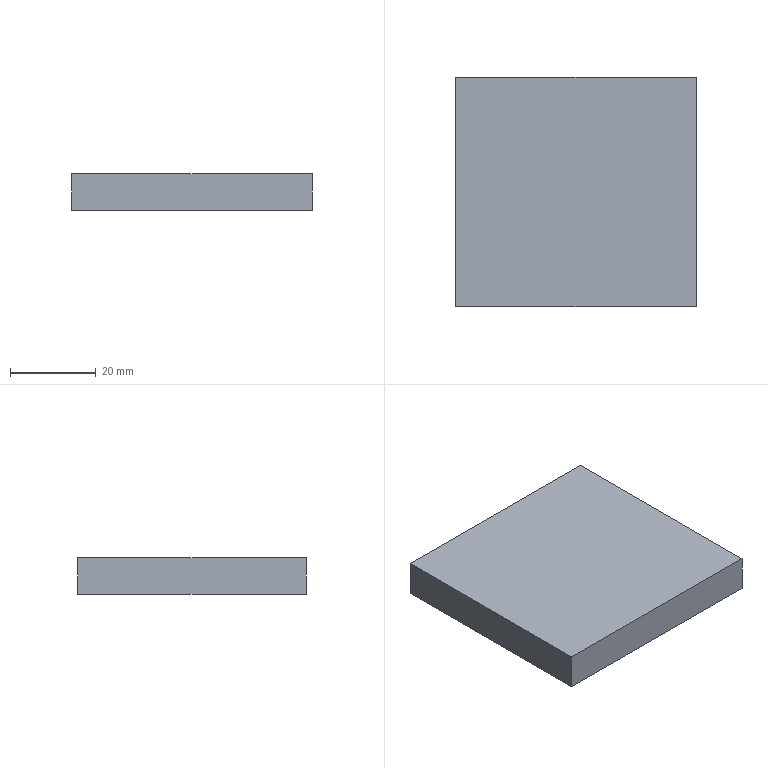NC program | NX | posted with a generic post | part box 56 x 53.3 x 8.5 mm
Lines 590 to 2012 of 2943:
(CAVITY_MILL_COPY_COPY , TOOL : D4)
N1178 T11 M6
N1180 G54
N1182 G17 G0 G90 X-8.53 Y16.809 S9500 M3
N1184 G43 Z30. H11
N1186 Z0.708
N1188 G94 G1 Z-0.292 F800.
N1190 X-8.86 Y16.999
N1192 G3 X-9.86 Y16.997 R1.
N1194 X-10.379 Y16.685 R19.65 F1200.
N1196 X-10.558 Y16.028 R0.5
N1198 G2 X-10.331 Y15.511 R4.05
N1200 G3 X-9.567 Y14.865 R1.
N1202 G1 X-9.34 Y14.824
N1204 Z0.708
N1206 X-8.53 Y16.809 Z0.417 F6000.
N1208 Z-0.583 F800.
N1210 X-8.86 Y16.999
N1212 G3 X-9.86 Y16.997 R1.
N1214 X-10.379 Y16.685 R19.65 F1200.
N1216 X-10.558 Y16.028 R0.5
N1218 G2 X-10.331 Y15.511 R4.05
N1220 G3 X-9.567 Y14.865 R1.
N1222 G1 X-9.34 Y14.824
N1224 Z0.417
N1226 X-8.53 Y16.809 Z0.125 F6000.
N1228 Z-0.875 F800.
N1230 X-8.86 Y16.999
N1232 G3 X-9.86 Y16.997 R1.
N1234 X-10.379 Y16.685 R19.65 F1200.
N1236 X-10.558 Y16.028 R0.5
N1238 G2 X-10.331 Y15.511 R4.05
N1240 G3 X-9.567 Y14.865 R1.
N1242 G1 X-9.34 Y14.824
N1244 Z0.125
N1246 X-8.53 Y16.809 Z-0.167 F6000.
N1248 Z-1.167 F800.
N1250 X-8.86 Y16.999
N1252 G3 X-9.86 Y16.997 R1.
N1254 X-10.379 Y16.685 R19.65 F1200.
N1256 X-10.558 Y16.028 R0.5
N1258 G2 X-10.331 Y15.511 R4.05
N1260 G3 X-9.567 Y14.865 R1.
N1262 G1 X-9.34 Y14.824
N1264 Z-0.167
N1266 X-8.53 Y16.809 Z-0.458 F6000.
N1268 Z-1.458 F800.
N1270 X-8.86 Y16.999
N1272 G3 X-9.86 Y16.997 R1.
N1274 X-10.379 Y16.685 R19.65 F1200.
N1276 X-10.558 Y16.028 R0.5
N1278 G2 X-10.331 Y15.511 R4.05
N1280 G3 X-9.567 Y14.865 R1.
N1282 G1 X-9.34 Y14.824
N1284 Z-0.458
N1286 X-8.53 Y16.809 Z-0.75 F6000.
N1288 Z-1.75 F800.
N1290 X-8.86 Y16.999
N1292 G3 X-9.86 Y16.997 R1.
N1294 X-10.379 Y16.685 R19.65 F1200.
N1296 X-10.558 Y16.028 R0.5
N1298 G2 X-10.331 Y15.511 R4.05
N1300 G3 X-9.567 Y14.865 R1.
N1302 G1 X-9.34 Y14.824
N1304 Z-0.75
N1306 X-8.53 Y16.809 Z-1.042 F6000.
N1308 Z-2.042 F800.
N1310 X-8.86 Y16.999
N1312 G3 X-9.86 Y16.997 R1.
N1314 X-10.379 Y16.685 R19.65 F1200.
N1316 X-10.558 Y16.028 R0.5
N1318 G2 X-10.331 Y15.511 R4.05
N1320 G3 X-9.567 Y14.865 R1.
N1322 G1 X-9.34 Y14.824
N1324 Z-1.042
N1326 X-8.53 Y16.809 Z-1.333 F6000.
N1328 Z-2.333 F800.
N1330 X-8.86 Y16.999
N1332 G3 X-9.86 Y16.997 R1.
N1334 X-10.379 Y16.685 R19.65 F1200.
N1336 X-10.558 Y16.028 R0.5
N1338 G2 X-10.331 Y15.511 R4.05
N1340 G3 X-9.567 Y14.865 R1.
N1342 G1 X-9.34 Y14.824
N1344 Z-1.333
N1346 X-8.53 Y16.809 Z-1.625 F6000.
N1348 Z-2.625 F800.
N1350 X-8.86 Y16.999
N1352 G3 X-9.86 Y16.997 R1.
N1354 X-10.379 Y16.685 R19.65 F1200.
N1356 X-10.558 Y16.028 R0.5
N1358 G2 X-10.331 Y15.511 R4.05
N1360 G3 X-9.567 Y14.865 R1.
N1362 G1 X-9.34 Y14.824
N1364 Z-1.625
N1366 X-8.53 Y16.809 Z-1.917 F6000.
N1368 Z-2.917 F800.
N1370 X-8.86 Y16.999
N1372 G3 X-9.86 Y16.997 R1.
N1374 X-10.379 Y16.685 R19.65 F1200.
N1376 X-10.558 Y16.028 R0.5
N1378 G2 X-10.331 Y15.511 R4.05
N1380 G3 X-9.567 Y14.865 R1.
N1382 G1 X-9.34 Y14.824
N1384 Z-1.917
N1386 X-8.53 Y16.809 Z-2.208 F6000.
N1388 Z-3.208 F800.
N1390 X-8.86 Y16.999
N1392 G3 X-9.86 Y16.997 R1.
N1394 X-10.379 Y16.685 R19.65 F1200.
N1396 X-10.558 Y16.028 R0.5
N1398 G2 X-10.331 Y15.511 R4.05
N1400 G3 X-9.567 Y14.865 R1.
N1402 G1 X-9.34 Y14.824
N1404 Z-2.208
N1406 X-8.53 Y16.809 Z-2.5 F6000.
N1408 Z-3.5 F800.
N1410 X-8.86 Y16.999
N1412 G3 X-9.86 Y16.997 R1.
N1414 X-10.379 Y16.685 R19.65 F1200.
N1416 X-10.558 Y16.028 R0.5
N1418 G2 X-10.331 Y15.511 R4.05
N1420 G3 X-9.567 Y14.865 R1.
N1422 G1 X-9.34 Y14.824
N1424 Z-2.5
N1426 G0 Z30.
N1428 X-14.824 Y9.34
N1430 Z0.708
N1432 G1 Z-0.292 F800.
N1434 X-14.865 Y9.567
N1436 G3 X-15.511 Y10.331 R1.
N1438 G2 X-16.028 Y10.558 R4.05 F1200.
N1440 G3 X-16.685 Y10.379 R0.5
N1442 X-16.997 Y9.86 R19.65
N1444 X-16.999 Y8.86 R1.
N1446 G1 X-16.809 Y8.53
N1448 Z0.708
N1450 X-14.824 Y9.34 Z0.417 F6000.
N1452 Z-0.583 F800.
N1454 X-14.865 Y9.567
N1456 G3 X-15.511 Y10.331 R1.
N1458 G2 X-16.028 Y10.558 R4.05 F1200.
N1460 G3 X-16.685 Y10.379 R0.5
N1462 X-16.997 Y9.86 R19.65
N1464 X-16.999 Y8.86 R1.
N1466 G1 X-16.809 Y8.53
N1468 Z0.417
N1470 X-14.824 Y9.34 Z0.125 F6000.
N1472 Z-0.875 F800.
N1474 X-14.865 Y9.567
N1476 G3 X-15.511 Y10.331 R1.
N1478 G2 X-16.028 Y10.558 R4.05 F1200.
N1480 G3 X-16.685 Y10.379 R0.5
N1482 X-16.997 Y9.86 R19.65
N1484 X-16.999 Y8.86 R1.
N1486 G1 X-16.809 Y8.53
N1488 Z0.125
N1490 X-14.824 Y9.34 Z-0.167 F6000.
N1492 Z-1.167 F800.
N1494 X-14.865 Y9.567
N1496 G3 X-15.511 Y10.331 R1.
N1498 G2 X-16.028 Y10.558 R4.05 F1200.
N1500 G3 X-16.685 Y10.379 R0.5
N1502 X-16.997 Y9.86 R19.65
N1504 X-16.999 Y8.86 R1.
N1506 G1 X-16.809 Y8.53
N1508 Z-0.167
N1510 X-14.824 Y9.34 Z-0.458 F6000.
N1512 Z-1.458 F800.
N1514 X-14.865 Y9.567
N1516 G3 X-15.511 Y10.331 R1.
N1518 G2 X-16.028 Y10.558 R4.05 F1200.
N1520 G3 X-16.685 Y10.379 R0.5
N1522 X-16.997 Y9.86 R19.65
N1524 X-16.999 Y8.86 R1.
N1526 G1 X-16.809 Y8.53
N1528 Z-0.458
N1530 X-14.824 Y9.34 Z-0.75 F6000.
N1532 Z-1.75 F800.
N1534 X-14.865 Y9.567
N1536 G3 X-15.511 Y10.331 R1.
N1538 G2 X-16.028 Y10.558 R4.05 F1200.
N1540 G3 X-16.685 Y10.379 R0.5
N1542 X-16.997 Y9.86 R19.65
N1544 X-16.999 Y8.86 R1.
N1546 G1 X-16.809 Y8.53
N1548 Z-0.75
N1550 X-14.824 Y9.34 Z-1.042 F6000.
N1552 Z-2.042 F800.
N1554 X-14.865 Y9.567
N1556 G3 X-15.511 Y10.331 R1.
N1558 G2 X-16.028 Y10.558 R4.05 F1200.
N1560 G3 X-16.685 Y10.379 R0.5
N1562 X-16.997 Y9.86 R19.65
N1564 X-16.999 Y8.86 R1.
N1566 G1 X-16.809 Y8.53
N1568 Z-1.042
N1570 X-14.824 Y9.34 Z-1.333 F6000.
N1572 Z-2.333 F800.
N1574 X-14.865 Y9.567
N1576 G3 X-15.511 Y10.331 R1.
N1578 G2 X-16.028 Y10.558 R4.05 F1200.
N1580 G3 X-16.685 Y10.379 R0.5
N1582 X-16.997 Y9.86 R19.65
N1584 X-16.999 Y8.86 R1.
N1586 G1 X-16.809 Y8.53
N1588 Z-1.333
N1590 X-14.824 Y9.34 Z-1.625 F6000.
N1592 Z-2.625 F800.
N1594 X-14.865 Y9.567
N1596 G3 X-15.511 Y10.331 R1.
N1598 G2 X-16.028 Y10.558 R4.05 F1200.
N1600 G3 X-16.685 Y10.379 R0.5
N1602 X-16.997 Y9.86 R19.65
N1604 X-16.999 Y8.86 R1.
N1606 G1 X-16.809 Y8.53
N1608 Z-1.625
N1610 X-14.824 Y9.34 Z-1.917 F6000.
N1612 Z-2.917 F800.
N1614 X-14.865 Y9.567
N1616 G3 X-15.511 Y10.331 R1.
N1618 G2 X-16.028 Y10.558 R4.05 F1200.
N1620 G3 X-16.685 Y10.379 R0.5
N1622 X-16.997 Y9.86 R19.65
N1624 X-16.999 Y8.86 R1.
N1626 G1 X-16.809 Y8.53
N1628 Z-1.917
N1630 X-14.824 Y9.34 Z-2.208 F6000.
N1632 Z-3.208 F800.
N1634 X-14.865 Y9.567
N1636 G3 X-15.511 Y10.331 R1.
N1638 G2 X-16.028 Y10.558 R4.05 F1200.
N1640 G3 X-16.685 Y10.379 R0.5
N1642 X-16.997 Y9.86 R19.65
N1644 X-16.999 Y8.86 R1.
N1646 G1 X-16.809 Y8.53
N1648 Z-2.208
N1650 X-14.824 Y9.34 Z-2.5 F6000.
N1652 Z-3.5 F800.
N1654 X-14.865 Y9.567
N1656 G3 X-15.511 Y10.331 R1.
N1658 G2 X-16.028 Y10.558 R4.05 F1200.
N1660 G3 X-16.685 Y10.379 R0.5
N1662 X-16.997 Y9.86 R19.65
N1664 X-16.999 Y8.86 R1.
N1666 G1 X-16.809 Y8.53
N1668 Z-2.5
N1670 G0 Z30.
N1672 X-18.46 Y5.669
N1674 Z0.708
N1676 G1 Z-0.292 F800.
N1678 X-18.629 Y5.779
N1680 G3 X-19.628 Y5.829 R1.
N1682 G2 X-20.241 Y5.596 R3. F1200.
N1684 G3 X-20.412 Y4.934 R21.
N1686 X-20.13 Y3.974 R1.
N1688 G1 X-19.856 Y3.713
N1690 Z0.708
N1692 X-18.46 Y5.669 Z0.417 F6000.
N1694 Z-0.583 F800.
N1696 X-18.629 Y5.779
N1698 G3 X-19.628 Y5.829 R1.
N1700 G2 X-20.241 Y5.596 R3. F1200.
N1702 G3 X-20.412 Y4.934 R21.
N1704 X-20.13 Y3.974 R1.
N1706 G1 X-19.856 Y3.713
N1708 Z0.417
N1710 X-18.46 Y5.669 Z0.125 F6000.
N1712 Z-0.875 F800.
N1714 X-18.629 Y5.779
N1716 G3 X-19.628 Y5.829 R1.
N1718 G2 X-20.241 Y5.596 R3. F1200.
N1720 G3 X-20.412 Y4.934 R21.
N1722 X-20.13 Y3.974 R1.
N1724 G1 X-19.856 Y3.713
N1726 Z0.125
N1728 X-18.46 Y5.669 Z-0.167 F6000.
N1730 Z-1.167 F800.
N1732 X-18.629 Y5.779
N1734 G3 X-19.628 Y5.829 R1.
N1736 G2 X-20.241 Y5.596 R3. F1200.
N1738 G3 X-20.412 Y4.934 R21.
N1740 X-20.13 Y3.974 R1.
N1742 G1 X-19.856 Y3.713
N1744 Z-0.167
N1746 X-18.46 Y5.669 Z-0.458 F6000.
N1748 Z-1.458 F800.
N1750 X-18.629 Y5.779
N1752 G3 X-19.628 Y5.829 R1.
N1754 G2 X-20.241 Y5.596 R3. F1200.
N1756 G3 X-20.412 Y4.934 R21.
N1758 X-20.13 Y3.974 R1.
N1760 G1 X-19.856 Y3.713
N1762 Z-0.458
N1764 X-18.46 Y5.669 Z-0.75 F6000.
N1766 Z-1.75 F800.
N1768 X-18.629 Y5.779
N1770 G3 X-19.628 Y5.829 R1.
N1772 G2 X-20.241 Y5.596 R3. F1200.
N1774 G3 X-20.412 Y4.934 R21.
N1776 X-20.13 Y3.974 R1.
N1778 G1 X-19.856 Y3.713
N1780 Z-0.75
N1782 X-18.46 Y5.669 Z-1.042 F6000.
N1784 Z-2.042 F800.
N1786 X-18.629 Y5.779
N1788 G3 X-19.628 Y5.829 R1.
N1790 G2 X-20.241 Y5.596 R3. F1200.
N1792 G3 X-20.412 Y4.934 R21.
N1794 X-20.13 Y3.974 R1.
N1796 G1 X-19.856 Y3.713
N1798 Z-1.042
N1800 X-18.46 Y5.669 Z-1.333 F6000.
N1802 Z-2.333 F800.
N1804 X-18.629 Y5.779
N1806 G3 X-19.628 Y5.829 R1.
N1808 G2 X-20.241 Y5.596 R3. F1200.
N1810 G3 X-20.412 Y4.934 R21.
N1812 X-20.13 Y3.974 R1.
N1814 G1 X-19.856 Y3.713
N1816 Z-1.333
N1818 X-18.46 Y5.669 Z-1.625 F6000.
N1820 Z-2.625 F800.
N1822 X-18.629 Y5.779
N1824 G3 X-19.628 Y5.829 R1.
N1826 G2 X-20.241 Y5.596 R3. F1200.
N1828 G3 X-20.412 Y4.934 R21.
N1830 X-20.13 Y3.974 R1.
N1832 G1 X-19.856 Y3.713
N1834 Z-1.625
N1836 X-18.46 Y5.669 Z-1.917 F6000.
N1838 Z-2.917 F800.
N1840 X-18.629 Y5.779
N1842 G3 X-19.628 Y5.829 R1.
N1844 G2 X-20.241 Y5.596 R3. F1200.
N1846 G3 X-20.412 Y4.934 R21.
N1848 X-20.13 Y3.974 R1.
N1850 G1 X-19.856 Y3.713
N1852 Z-1.917
N1854 X-18.46 Y5.669 Z-2.208 F6000.
N1856 Z-3.208 F800.
N1858 X-18.629 Y5.779
N1860 G3 X-19.628 Y5.829 R1.
N1862 G2 X-20.241 Y5.596 R3. F1200.
N1864 G3 X-20.412 Y4.934 R21.
N1866 X-20.13 Y3.974 R1.
N1868 G1 X-19.856 Y3.713
N1870 Z-2.208
N1872 X-18.46 Y5.669 Z-2.5 F6000.
N1874 Z-3.5 F800.
N1876 X-18.629 Y5.779
N1878 G3 X-19.628 Y5.829 R1.
N1880 G2 X-20.241 Y5.596 R3. F1200.
N1882 G3 X-20.412 Y4.934 R21.
N1884 X-20.13 Y3.974 R1.
N1886 G1 X-19.856 Y3.713
N1888 Z-2.5
N1890 G0 Z30.
N1892 Y-3.713
N1894 Z0.708
N1896 G1 Z-0.292 F800.
N1898 X-20.13 Y-3.974
N1900 G3 X-20.412 Y-4.934 R1.
N1902 X-20.241 Y-5.596 R21. F1200.
N1904 G2 X-19.628 Y-5.829 R3.
N1906 G3 X-18.629 Y-5.779 R1.
N1908 G1 X-18.46 Y-5.669
N1910 Z0.708
N1912 X-19.856 Y-3.713 Z0.417 F6000.
N1914 Z-0.583 F800.
N1916 X-20.13 Y-3.974
N1918 G3 X-20.412 Y-4.934 R1.
N1920 X-20.241 Y-5.596 R21. F1200.
N1922 G2 X-19.628 Y-5.829 R3.
N1924 G3 X-18.629 Y-5.779 R1.
N1926 G1 X-18.46 Y-5.669
N1928 Z0.417
N1930 X-19.856 Y-3.713 Z0.125 F6000.
N1932 Z-0.875 F800.
N1934 X-20.13 Y-3.974
N1936 G3 X-20.412 Y-4.934 R1.
N1938 X-20.241 Y-5.596 R21. F1200.
N1940 G2 X-19.628 Y-5.829 R3.
N1942 G3 X-18.629 Y-5.779 R1.
N1944 G1 X-18.46 Y-5.669
N1946 Z0.125
N1948 X-19.856 Y-3.713 Z-0.167 F6000.
N1950 Z-1.167 F800.
N1952 X-20.13 Y-3.974
N1954 G3 X-20.412 Y-4.934 R1.
N1956 X-20.241 Y-5.596 R21. F1200.
N1958 G2 X-19.628 Y-5.829 R3.
N1960 G3 X-18.629 Y-5.779 R1.
N1962 G1 X-18.46 Y-5.669
N1964 Z-0.167
N1966 X-19.856 Y-3.713 Z-0.458 F6000.
N1968 Z-1.458 F800.
N1970 X-20.13 Y-3.974
N1972 G3 X-20.412 Y-4.934 R1.
N1974 X-20.241 Y-5.596 R21. F1200.
N1976 G2 X-19.628 Y-5.829 R3.
N1978 G3 X-18.629 Y-5.779 R1.
N1980 G1 X-18.46 Y-5.669
N1982 Z-0.458
N1984 X-19.856 Y-3.713 Z-0.75 F6000.
N1986 Z-1.75 F800.
N1988 X-20.13 Y-3.974
N1990 G3 X-20.412 Y-4.934 R1.
N1992 X-20.241 Y-5.596 R21. F1200.
N1994 G2 X-19.628 Y-5.829 R3.
N1996 G3 X-18.629 Y-5.779 R1.
N1998 G1 X-18.46 Y-5.669
N2000 Z-0.75
N2002 X-19.856 Y-3.713 Z-1.042 F6000.
N2004 Z-2.042 F800.
N2006 X-20.13 Y-3.974
N2008 G3 X-20.412 Y-4.934 R1.
N2010 X-20.241 Y-5.596 R21. F1200.
N2012 G2 X-19.628 Y-5.829 R3.
N2014 G3 X-18.629 Y-5.779 R1.
N2016 G1 X-18.46 Y-5.669
N2018 Z-1.042
N2020 X-19.856 Y-3.713 Z-1.333 F6000.
N2022 Z-2.333 F800.
N2024 X-20.13 Y-3.974
N2026 G3 X-20.412 Y-4.934 R1.
N2028 X-20.241 Y-5.596 R21. F1200.
N2030 G2 X-19.628 Y-5.829 R3.
N2032 G3 X-18.629 Y-5.779 R1.
N2034 G1 X-18.46 Y-5.669
N2036 Z-1.333
N2038 X-19.856 Y-3.713 Z-1.625 F6000.
N2040 Z-2.625 F800.
N2042 X-20.13 Y-3.974
N2044 G3 X-20.412 Y-4.934 R1.
N2046 X-20.241 Y-5.596 R21. F1200.
N2048 G2 X-19.628 Y-5.829 R3.
N2050 G3 X-18.629 Y-5.779 R1.
N2052 G1 X-18.46 Y-5.669
N2054 Z-1.625
N2056 X-19.856 Y-3.713 Z-1.917 F6000.
N2058 Z-2.917 F800.
N2060 X-20.13 Y-3.974
N2062 G3 X-20.412 Y-4.934 R1.
N2064 X-20.241 Y-5.596 R21. F1200.
N2066 G2 X-19.628 Y-5.829 R3.
N2068 G3 X-18.629 Y-5.779 R1.
N2070 G1 X-18.46 Y-5.669
N2072 Z-1.917
N2074 X-19.856 Y-3.713 Z-2.208 F6000.
N2076 Z-3.208 F800.
N2078 X-20.13 Y-3.974
N2080 G3 X-20.412 Y-4.934 R1.
N2082 X-20.241 Y-5.596 R21. F1200.
N2084 G2 X-19.628 Y-5.829 R3.
N2086 G3 X-18.629 Y-5.779 R1.
N2088 G1 X-18.46 Y-5.669
N2090 Z-2.208
N2092 X-19.856 Y-3.713 Z-2.5 F6000.
N2094 Z-3.5 F800.
N2096 X-20.13 Y-3.974
N2098 G3 X-20.412 Y-4.934 R1.
N2100 X-20.241 Y-5.596 R21. F1200.
N2102 G2 X-19.628 Y-5.829 R3.
N2104 G3 X-18.629 Y-5.779 R1.
N2106 G1 X-18.46 Y-5.669
N2108 Z-2.5
N2110 G0 Z30.
N2112 X-16.809 Y-8.53
N2114 Z0.708
N2116 G1 Z-0.292 F800.
N2118 X-16.999 Y-8.86
N2120 G3 X-16.997 Y-9.86 R1.
N2122 X-16.685 Y-10.379 R19.65 F1200.
N2124 X-16.028 Y-10.558 R0.5
N2126 G2 X-15.511 Y-10.331 R4.05
N2128 G3 X-14.865 Y-9.567 R1.
N2130 G1 X-14.824 Y-9.34
N2132 Z0.708
N2134 X-16.809 Y-8.53 Z0.417 F6000.
N2136 Z-0.583 F800.
N2138 X-16.999 Y-8.86
N2140 G3 X-16.997 Y-9.86 R1.
N2142 X-16.685 Y-10.379 R19.65 F1200.
N2144 X-16.028 Y-10.558 R0.5
N2146 G2 X-15.511 Y-10.331 R4.05
N2148 G3 X-14.865 Y-9.567 R1.
N2150 G1 X-14.824 Y-9.34
N2152 Z0.417
N2154 X-16.809 Y-8.53 Z0.125 F6000.
N2156 Z-0.875 F800.
N2158 X-16.999 Y-8.86
N2160 G3 X-16.997 Y-9.86 R1.
N2162 X-16.685 Y-10.379 R19.65 F1200.
N2164 X-16.028 Y-10.558 R0.5
N2166 G2 X-15.511 Y-10.331 R4.05
N2168 G3 X-14.865 Y-9.567 R1.
N2170 G1 X-14.824 Y-9.34
N2172 Z0.125
N2174 X-16.809 Y-8.53 Z-0.167 F6000.
N2176 Z-1.167 F800.
N2178 X-16.999 Y-8.86
N2180 G3 X-16.997 Y-9.86 R1.
N2182 X-16.685 Y-10.379 R19.65 F1200.
N2184 X-16.028 Y-10.558 R0.5
N2186 G2 X-15.511 Y-10.331 R4.05
N2188 G3 X-14.865 Y-9.567 R1.
N2190 G1 X-14.824 Y-9.34
N2192 Z-0.167
N2194 X-16.809 Y-8.53 Z-0.458 F6000.
N2196 Z-1.458 F800.
N2198 X-16.999 Y-8.86
N2200 G3 X-16.997 Y-9.86 R1.
N2202 X-16.685 Y-10.379 R19.65 F1200.
N2204 X-16.028 Y-10.558 R0.5
N2206 G2 X-15.511 Y-10.331 R4.05
N2208 G3 X-14.865 Y-9.567 R1.
N2210 G1 X-14.824 Y-9.34
N2212 Z-0.458
N2214 X-16.809 Y-8.53 Z-0.75 F6000.
N2216 Z-1.75 F800.
N2218 X-16.999 Y-8.86
N2220 G3 X-16.997 Y-9.86 R1.
N2222 X-16.685 Y-10.379 R19.65 F1200.
N2224 X-16.028 Y-10.558 R0.5
N2226 G2 X-15.511 Y-10.331 R4.05
N2228 G3 X-14.865 Y-9.567 R1.
N2230 G1 X-14.824 Y-9.34
N2232 Z-0.75
N2234 X-16.809 Y-8.53 Z-1.042 F6000.
N2236 Z-2.042 F800.
N2238 X-16.999 Y-8.86
N2240 G3 X-16.997 Y-9.86 R1.
N2242 X-16.685 Y-10.379 R19.65 F1200.
N2244 X-16.028 Y-10.558 R0.5
N2246 G2 X-15.511 Y-10.331 R4.05
N2248 G3 X-14.865 Y-9.567 R1.
N2250 G1 X-14.824 Y-9.34
N2252 Z-1.042
N2254 X-16.809 Y-8.53 Z-1.333 F6000.
N2256 Z-2.333 F800.
N2258 X-16.999 Y-8.86
N2260 G3 X-16.997 Y-9.86 R1.
N2262 X-16.685 Y-10.379 R19.65 F1200.
N2264 X-16.028 Y-10.558 R0.5
N2266 G2 X-15.511 Y-10.331 R4.05
N2268 G3 X-14.865 Y-9.567 R1.
N2270 G1 X-14.824 Y-9.34
N2272 Z-1.333
N2274 X-16.809 Y-8.53 Z-1.625 F6000.
N2276 Z-2.625 F800.
N2278 X-16.999 Y-8.86
N2280 G3 X-16.997 Y-9.86 R1.
N2282 X-16.685 Y-10.379 R19.65 F1200.
N2284 X-16.028 Y-10.558 R0.5
N2286 G2 X-15.511 Y-10.331 R4.05
N2288 G3 X-14.865 Y-9.567 R1.
N2290 G1 X-14.824 Y-9.34
N2292 Z-1.625
N2294 X-16.809 Y-8.53 Z-1.917 F6000.
N2296 Z-2.917 F800.
N2298 X-16.999 Y-8.86
N2300 G3 X-16.997 Y-9.86 R1.
N2302 X-16.685 Y-10.379 R19.65 F1200.
N2304 X-16.028 Y-10.558 R0.5
N2306 G2 X-15.511 Y-10.331 R4.05
N2308 G3 X-14.865 Y-9.567 R1.
N2310 G1 X-14.824 Y-9.34
N2312 Z-1.917
N2314 X-16.809 Y-8.53 Z-2.208 F6000.
N2316 Z-3.208 F800.
N2318 X-16.999 Y-8.86
N2320 G3 X-16.997 Y-9.86 R1.
N2322 X-16.685 Y-10.379 R19.65 F1200.
N2324 X-16.028 Y-10.558 R0.5
N2326 G2 X-15.511 Y-10.331 R4.05
N2328 G3 X-14.865 Y-9.567 R1.
N2330 G1 X-14.824 Y-9.34
N2332 Z-2.208
N2334 X-16.809 Y-8.53 Z-2.5 F6000.
N2336 Z-3.5 F800.
N2338 X-16.999 Y-8.86
N2340 G3 X-16.997 Y-9.86 R1.
N2342 X-16.685 Y-10.379 R19.65 F1200.
N2344 X-16.028 Y-10.558 R0.5
N2346 G2 X-15.511 Y-10.331 R4.05
N2348 G3 X-14.865 Y-9.567 R1.
N2350 G1 X-14.824 Y-9.34
N2352 Z-2.5
N2354 G0 Z30.
N2356 X-9.34 Y-14.824
N2358 Z0.708
N2360 G1 Z-0.292 F800.
N2362 X-9.567 Y-14.865
N2364 G3 X-10.331 Y-15.511 R1.
N2366 G2 X-10.558 Y-16.028 R4.05 F1200.
N2368 G3 X-10.379 Y-16.685 R0.5
N2370 X-9.86 Y-16.997 R19.65
N2372 X-8.86 Y-16.999 R1.
N2374 G1 X-8.53 Y-16.809
N2376 Z0.708
N2378 X-9.34 Y-14.824 Z0.417 F6000.
N2380 Z-0.583 F800.
N2382 X-9.567 Y-14.865
N2384 G3 X-10.331 Y-15.511 R1.
N2386 G2 X-10.558 Y-16.028 R4.05 F1200.
N2388 G3 X-10.379 Y-16.685 R0.5
N2390 X-9.86 Y-16.997 R19.65
N2392 X-8.86 Y-16.999 R1.
N2394 G1 X-8.53 Y-16.81
N2396 Z0.417
N2398 X-9.34 Y-14.824 Z0.125 F6000.
N2400 Z-0.875 F800.
N2402 X-9.567 Y-14.865
N2404 G3 X-10.331 Y-15.511 R1.
N2406 G2 X-10.558 Y-16.028 R4.05 F1200.
N2408 G3 X-10.379 Y-16.685 R0.5
N2410 X-9.86 Y-16.997 R19.65
N2412 X-8.86 Y-16.999 R1.
N2414 G1 X-8.53 Y-16.81
N2416 Z0.125
N2418 X-9.34 Y-14.824 Z-0.167 F6000.
N2420 Z-1.167 F800.
N2422 X-9.567 Y-14.865
N2424 G3 X-10.331 Y-15.511 R1.
N2426 G2 X-10.558 Y-16.028 R4.05 F1200.
N2428 G3 X-10.379 Y-16.685 R0.5
N2430 X-9.86 Y-16.997 R19.65
N2432 X-8.86 Y-16.999 R1.
N2434 G1 X-8.53 Y-16.81
N2436 Z-0.167
N2438 X-9.34 Y-14.824 Z-0.458 F6000.
N2440 Z-1.458 F800.
N2442 X-9.567 Y-14.865
N2444 G3 X-10.33 Y-15.511 R1.
N2446 G2 X-10.558 Y-16.028 R4.05 F1200.
N2448 G3 X-10.379 Y-16.685 R0.5
N2450 X-9.86 Y-16.997 R19.65
N2452 X-8.86 Y-16.999 R1.
N2454 G1 X-8.53 Y-16.81
N2456 Z-0.458
N2458 X-9.34 Y-14.824 Z-0.75 F6000.
N2460 Z-1.75 F800.
N2462 X-9.567 Y-14.865
N2464 G3 X-10.33 Y-15.511 R1.
N2466 G2 X-10.558 Y-16.028 R4.05 F1200.
N2468 G3 X-10.379 Y-16.685 R0.5
N2470 X-9.86 Y-16.997 R19.65
N2472 X-8.86 Y-16.999 R1.
N2474 G1 X-8.53 Y-16.81
N2476 Z-0.75
N2478 X-9.34 Y-14.824 Z-1.042 F6000.
N2480 Z-2.042 F800.
N2482 X-9.567 Y-14.865
N2484 G3 X-10.33 Y-15.511 R1.
N2486 G2 X-10.558 Y-16.028 R4.05 F1200.
N2488 G3 X-10.379 Y-16.685 R0.5
N2490 X-9.86 Y-16.997 R19.65
N2492 X-8.86 Y-16.999 R1.
N2494 G1 X-8.53 Y-16.81
N2496 Z-1.042
N2498 X-9.34 Y-14.824 Z-1.333 F6000.
N2500 Z-2.333 F800.
N2502 X-9.567 Y-14.865
N2504 G3 X-10.33 Y-15.511 R1.
N2506 G2 X-10.558 Y-16.028 R4.05 F1200.
N2508 G3 X-10.379 Y-16.685 R0.5
N2510 X-9.86 Y-16.997 R19.65
N2512 X-8.86 Y-16.999 R1.
N2514 G1 X-8.53 Y-16.81
N2516 Z-1.333
N2518 X-9.34 Y-14.823 Z-1.625 F6000.
N2520 Z-2.625 F800.
N2522 X-9.567 Y-14.864
N2524 G3 X-10.33 Y-15.511 R1.
N2526 G2 X-10.558 Y-16.028 R4.05 F1200.
N2528 G3 X-10.379 Y-16.685 R0.5
N2530 X-9.859 Y-16.997 R19.65
N2532 X-8.859 Y-16.999 R1.
N2534 G1 X-8.529 Y-16.81
N2536 Z-1.625
N2538 X-9.34 Y-14.823 Z-1.917 F6000.
N2540 Z-2.917 F800.
N2542 X-9.567 Y-14.864
N2544 G3 X-10.33 Y-15.511 R1.
N2546 G2 X-10.558 Y-16.028 R4.05 F1200.
N2548 G3 X-10.379 Y-16.685 R0.5
N2550 X-9.859 Y-16.998 R19.65
N2552 X-8.859 Y-17. R1.
N2554 G1 X-8.529 Y-16.81
N2556 Z-1.917
N2558 X-9.34 Y-14.823 Z-2.208 F6000.
N2560 Z-3.208 F800.
N2562 X-9.567 Y-14.864
N2564 G3 X-10.33 Y-15.51 R1.
N2566 G2 X-10.558 Y-16.028 R4.05 F1200.
N2568 G3 X-10.379 Y-16.685 R0.5
N2570 X-9.859 Y-16.998 R19.65
N2572 X-8.859 Y-17. R1.
N2574 G1 X-8.529 Y-16.81
N2576 Z-2.208
N2578 X-9.34 Y-14.823 Z-2.5 F6000.
N2580 Z-3.5 F800.
N2582 X-9.567 Y-14.864
N2584 G3 X-10.33 Y-15.51 R1.
N2586 G2 X-10.558 Y-16.028 R4.05 F1200.
N2588 G3 X-10.379 Y-16.685 R0.5
N2590 X-9.859 Y-16.998 R19.65
N2592 X-8.859 Y-17. R1.
N2594 G1 X-8.529 Y-16.81
N2596 Z-2.5
N2598 G0 Z30.
N2600 X8.53 Y-16.809
N2602 Z0.708
N2604 G1 Z-0.292 F800.
N2606 X8.86 Y-16.999
N2608 G3 X9.86 Y-16.997 R1.
N2610 X10.379 Y-16.685 R19.65 F1200.
N2612 X10.558 Y-16.028 R0.5
N2614 G2 X10.331 Y-15.511 R4.05
N2616 G3 X9.567 Y-14.865 R1.
N2618 G1 X9.34 Y-14.824
N2620 Z0.708
N2622 X8.53 Y-16.809 Z0.417 F6000.
N2624 Z-0.583 F800.
N2626 X8.86 Y-16.999
N2628 G3 X9.86 Y-16.997 R1.
N2630 X10.379 Y-16.685 R19.65 F1200.
N2632 X10.558 Y-16.028 R0.5
N2634 G2 X10.331 Y-15.511 R4.05
N2636 G3 X9.567 Y-14.865 R1.
N2638 G1 X9.34 Y-14.824
N2640 Z0.417
N2642 X8.53 Y-16.809 Z0.125 F6000.
N2644 Z-0.875 F800.
N2646 X8.86 Y-16.999
N2648 G3 X9.86 Y-16.997 R1.
N2650 X10.379 Y-16.685 R19.65 F1200.
N2652 X10.558 Y-16.028 R0.5
N2654 G2 X10.331 Y-15.511 R4.05
N2656 G3 X9.567 Y-14.865 R1.
N2658 G1 X9.34 Y-14.824
N2660 Z0.125
N2662 X8.53 Y-16.809 Z-0.167 F6000.
N2664 Z-1.167 F800.
N2666 X8.86 Y-16.999
N2668 G3 X9.86 Y-16.997 R1.
N2670 X10.379 Y-16.685 R19.65 F1200.
N2672 X10.558 Y-16.028 R0.5
N2674 G2 X10.331 Y-15.511 R4.05
N2676 G3 X9.567 Y-14.865 R1.
N2678 G1 X9.34 Y-14.824
N2680 Z-0.167
N2682 X8.53 Y-16.809 Z-0.458 F6000.
N2684 Z-1.458 F800.
N2686 X8.86 Y-16.999
N2688 G3 X9.86 Y-16.997 R1.
N2690 X10.379 Y-16.685 R19.65 F1200.
N2692 X10.558 Y-16.028 R0.5
N2694 G2 X10.331 Y-15.511 R4.05
N2696 G3 X9.567 Y-14.865 R1.
N2698 G1 X9.34 Y-14.824
N2700 Z-0.458
N2702 X8.53 Y-16.809 Z-0.75 F6000.
N2704 Z-1.75 F800.
N2706 X8.86 Y-16.999
N2708 G3 X9.86 Y-16.997 R1.
N2710 X10.379 Y-16.685 R19.65 F1200.
N2712 X10.558 Y-16.028 R0.5
N2714 G2 X10.331 Y-15.511 R4.05
N2716 G3 X9.567 Y-14.865 R1.
N2718 G1 X9.34 Y-14.824
N2720 Z-0.75
N2722 X8.53 Y-16.809 Z-1.042 F6000.
N2724 Z-2.042 F800.
N2726 X8.86 Y-16.999
N2728 G3 X9.86 Y-16.997 R1.
N2730 X10.379 Y-16.685 R19.65 F1200.
N2732 X10.558 Y-16.028 R0.5
N2734 G2 X10.331 Y-15.511 R4.05
N2736 G3 X9.567 Y-14.865 R1.
N2738 G1 X9.34 Y-14.824
N2740 Z-1.042
N2742 X8.53 Y-16.809 Z-1.333 F6000.
N2744 Z-2.333 F800.
N2746 X8.86 Y-16.999
N2748 G3 X9.86 Y-16.997 R1.
N2750 X10.379 Y-16.685 R19.65 F1200.
N2752 X10.558 Y-16.028 R0.5
N2754 G2 X10.331 Y-15.511 R4.05
N2756 G3 X9.567 Y-14.865 R1.
N2758 G1 X9.34 Y-14.824
N2760 Z-1.333
N2762 X8.53 Y-16.809 Z-1.625 F6000.
N2764 Z-2.625 F800.
N2766 X8.86 Y-16.999
N2768 G3 X9.86 Y-16.997 R1.
N2770 X10.379 Y-16.685 R19.65 F1200.
N2772 X10.558 Y-16.028 R0.5
N2774 G2 X10.331 Y-15.511 R4.05
N2776 G3 X9.567 Y-14.865 R1.
N2778 G1 X9.34 Y-14.824
N2780 Z-1.625
N2782 X8.53 Y-16.809 Z-1.917 F6000.
N2784 Z-2.917 F800.
N2786 X8.86 Y-16.999
N2788 G3 X9.86 Y-16.997 R1.
N2790 X10.379 Y-16.685 R19.65 F1200.
N2792 X10.558 Y-16.028 R0.5
N2794 G2 X10.331 Y-15.511 R4.05
N2796 G3 X9.567 Y-14.865 R1.
N2798 G1 X9.34 Y-14.824
N2800 Z-1.917
N2802 X8.53 Y-16.809 Z-2.208 F6000.
N2804 Z-3.208 F800.
N2806 X8.86 Y-16.999
N2808 G3 X9.86 Y-16.997 R1.
N2810 X10.379 Y-16.685 R19.65 F1200.
N2812 X10.558 Y-16.028 R0.5
N2814 G2 X10.331 Y-15.511 R4.05
N2816 G3 X9.567 Y-14.865 R1.
N2818 G1 X9.34 Y-14.824
N2820 Z-2.208
N2822 X8.53 Y-16.809 Z-2.5 F6000.
N2824 Z-3.5 F800.
N2826 X8.86 Y-16.999
N2828 G3 X9.86 Y-16.997 R1.
N2830 X10.379 Y-16.685 R19.65 F1200.
N2832 X10.558 Y-16.028 R0.5
N2834 G2 X10.331 Y-15.511 R4.05
N2836 G3 X9.567 Y-14.865 R1.
N2838 G1 X9.34 Y-14.824
N2840 Z-2.5
N2842 G0 Z30.
N2844 X14.824 Y-9.34
N2846 Z0.708
N2848 G1 Z-0.292 F800.
N2850 X14.865 Y-9.567
N2852 G3 X15.511 Y-10.331 R1.
N2854 G2 X16.028 Y-10.558 R4.05 F1200.
N2856 G3 X16.685 Y-10.379 R0.5
N2858 X16.997 Y-9.86 R19.65
N2860 X16.999 Y-8.86 R1.
N2862 G1 X16.809 Y-8.53
N2864 Z0.708
N2866 X14.824 Y-9.34 Z0.417 F6000.
N2868 Z-0.583 F800.
N2870 X14.865 Y-9.567
N2872 G3 X15.511 Y-10.331 R1.
N2874 G2 X16.028 Y-10.558 R4.05 F1200.
N2876 G3 X16.685 Y-10.379 R0.5
N2878 X16.997 Y-9.86 R19.65
N2880 X16.999 Y-8.86 R1.
N2882 G1 X16.809 Y-8.53
N2884 Z0.417
N2886 X14.824 Y-9.34 Z0.125 F6000.
N2888 Z-0.875 F800.
N2890 X14.865 Y-9.567
N2892 G3 X15.511 Y-10.331 R1.
N2894 G2 X16.028 Y-10.558 R4.05 F1200.
N2896 G3 X16.685 Y-10.379 R0.5
N2898 X16.997 Y-9.86 R19.65
N2900 X16.999 Y-8.86 R1.
N2902 G1 X16.809 Y-8.53
N2904 Z0.125
N2906 X14.824 Y-9.34 Z-0.167 F6000.
N2908 Z-1.167 F800.
N2910 X14.865 Y-9.567
N2912 G3 X15.511 Y-10.331 R1.
N2914 G2 X16.028 Y-10.558 R4.05 F1200.
N2916 G3 X16.685 Y-10.379 R0.5
N2918 X16.997 Y-9.86 R19.65
N2920 X16.999 Y-8.86 R1.
N2922 G1 X16.809 Y-8.53
N2924 Z-0.167
N2926 X14.824 Y-9.34 Z-0.458 F6000.
N2928 Z-1.458 F800.
N2930 X14.865 Y-9.567
N2932 G3 X15.511 Y-10.331 R1.
N2934 G2 X16.028 Y-10.558 R4.05 F1200.
N2936 G3 X16.685 Y-10.379 R0.5
N2938 X16.997 Y-9.86 R19.65
N2940 X16.999 Y-8.86 R1.
N2942 G1 X16.809 Y-8.53
N2944 Z-0.458
N2946 X14.824 Y-9.34 Z-0.75 F6000.
N2948 Z-1.75 F800.
N2950 X14.865 Y-9.567
N2952 G3 X15.511 Y-10.331 R1.
N2954 G2 X16.028 Y-10.558 R4.05 F1200.
N2956 G3 X16.685 Y-10.379 R0.5
N2958 X16.997 Y-9.86 R19.65
N2960 X16.999 Y-8.86 R1.
N2962 G1 X16.809 Y-8.53
N2964 Z-0.75
N2966 X14.824 Y-9.34 Z-1.042 F6000.
N2968 Z-2.042 F800.
N2970 X14.865 Y-9.567
N2972 G3 X15.511 Y-10.331 R1.
N2974 G2 X16.028 Y-10.558 R4.05 F1200.
N2976 G3 X16.685 Y-10.379 R0.5
N2978 X16.997 Y-9.86 R19.65
N2980 X16.999 Y-8.86 R1.
N2982 G1 X16.809 Y-8.53
N2984 Z-1.042
N2986 X14.824 Y-9.34 Z-1.333 F6000.
N2988 Z-2.333 F800.
N2990 X14.865 Y-9.567
N2992 G3 X15.511 Y-10.331 R1.
N2994 G2 X16.028 Y-10.558 R4.05 F1200.
N2996 G3 X16.685 Y-10.379 R0.5
N2998 X16.997 Y-9.86 R19.65
N3000 X16.999 Y-8.86 R1.
N3002 G1 X16.809 Y-8.53
N3004 Z-1.333
N3006 X14.824 Y-9.34 Z-1.625 F6000.
N3008 Z-2.625 F800.
N3010 X14.865 Y-9.567
N3012 G3 X15.511 Y-10.331 R1.
N3014 G2 X16.028 Y-10.558 R4.05 F1200.
N3016 G3 X16.685 Y-10.379 R0.5
N3018 X16.997 Y-9.86 R19.65
N3020 X16.999 Y-8.86 R1.
N3022 G1 X16.809 Y-8.53
N3024 Z-1.625
N3026 X14.824 Y-9.34 Z-1.917 F6000.
N3028 Z-2.917 F800.
N3030 X14.865 Y-9.567
N3032 G3 X15.511 Y-10.331 R1.
N3034 G2 X16.028 Y-10.558 R4.05 F1200.
N3036 G3 X16.685 Y-10.379 R0.5
N3038 X16.997 Y-9.86 R19.65
N3040 X16.999 Y-8.86 R1.
N3042 G1 X16.809 Y-8.53
N3044 Z-1.917
N3046 X14.824 Y-9.34 Z-2.208 F6000.
N3048 Z-3.208 F800.
N3050 X14.865 Y-9.567
N3052 G3 X15.511 Y-10.331 R1.
N3054 G2 X16.028 Y-10.558 R4.05 F1200.
N3056 G3 X16.685 Y-10.379 R0.5
N3058 X16.997 Y-9.86 R19.65
N3060 X16.999 Y-8.86 R1.
N3062 G1 X16.809 Y-8.53
N3064 Z-2.208
N3066 X14.824 Y-9.34 Z-2.5 F6000.
N3068 Z-3.5 F800.
N3070 X14.865 Y-9.567
N3072 G3 X15.511 Y-10.331 R1.
N3074 G2 X16.028 Y-10.558 R4.05 F1200.
N3076 G3 X16.685 Y-10.379 R0.5
N3078 X16.997 Y-9.86 R19.65
N3080 X16.999 Y-8.86 R1.
N3082 G1 X16.809 Y-8.53
N3084 Z-2.5
N3086 G0 Z30.
N3088 X18.46 Y-5.669
N3090 Z0.708
N3092 G1 Z-0.292 F800.
N3094 X18.629 Y-5.779
N3096 G3 X19.628 Y-5.829 R1.
N3098 G2 X20.241 Y-5.596 R3. F1200.
N3100 G3 X20.412 Y-4.934 R21.
N3102 X20.13 Y-3.974 R1.
N3104 G1 X19.856 Y-3.713
N3106 Z0.708
N3108 X18.46 Y-5.669 Z0.417 F6000.
N3110 Z-0.583 F800.
N3112 X18.629 Y-5.779
N3114 G3 X19.628 Y-5.829 R1.
N3116 G2 X20.241 Y-5.596 R3. F1200.
N3118 G3 X20.412 Y-4.934 R21.
N3120 X20.13 Y-3.974 R1.
N3122 G1 X19.856 Y-3.713
N3124 Z0.417
N3126 X18.46 Y-5.669 Z0.125 F6000.
N3128 Z-0.875 F800.
N3130 X18.629 Y-5.779
N3132 G3 X19.628 Y-5.829 R1.
N3134 G2 X20.241 Y-5.596 R3. F1200.
N3136 G3 X20.412 Y-4.934 R21.
N3138 X20.13 Y-3.974 R1.
N3140 G1 X19.856 Y-3.713
N3142 Z0.125
N3144 X18.46 Y-5.669 Z-0.167 F6000.
N3146 Z-1.167 F800.
N3148 X18.629 Y-5.779
N3150 G3 X19.628 Y-5.829 R1.
N3152 G2 X20.241 Y-5.596 R3. F1200.
N3154 G3 X20.412 Y-4.934 R21.
N3156 X20.13 Y-3.974 R1.
N3158 G1 X19.856 Y-3.713
N3160 Z-0.167
N3162 X18.46 Y-5.669 Z-0.458 F6000.
N3164 Z-1.458 F800.
N3166 X18.629 Y-5.779
N3168 G3 X19.628 Y-5.829 R1.
N3170 G2 X20.241 Y-5.596 R3. F1200.
N3172 G3 X20.412 Y-4.934 R21.
N3174 X20.13 Y-3.974 R1.
N3176 G1 X19.856 Y-3.713
N3178 Z-0.458
N3180 X18.46 Y-5.669 Z-0.75 F6000.
N3182 Z-1.75 F800.
N3184 X18.629 Y-5.779
N3186 G3 X19.628 Y-5.829 R1.
N3188 G2 X20.241 Y-5.596 R3. F1200.
N3190 G3 X20.412 Y-4.934 R21.
N3192 X20.13 Y-3.974 R1.
N3194 G1 X19.856 Y-3.713
N3196 Z-0.75
N3198 X18.46 Y-5.669 Z-1.042 F6000.
N3200 Z-2.042 F800.
N3202 X18.629 Y-5.779
N3204 G3 X19.628 Y-5.829 R1.
N3206 G2 X20.241 Y-5.596 R3. F1200.
N3208 G3 X20.412 Y-4.934 R21.
N3210 X20.13 Y-3.974 R1.
N3212 G1 X19.856 Y-3.713
N3214 Z-1.042
N3216 X18.46 Y-5.669 Z-1.333 F6000.
N3218 Z-2.333 F800.
N3220 X18.629 Y-5.779
N3222 G3 X19.628 Y-5.829 R1.
N3224 G2 X20.241 Y-5.596 R3. F1200.
N3226 G3 X20.412 Y-4.934 R21.
N3228 X20.13 Y-3.974 R1.
N3230 G1 X19.856 Y-3.713
N3232 Z-1.333
N3234 X18.46 Y-5.669 Z-1.625 F6000.
N3236 Z-2.625 F800.
N3238 X18.629 Y-5.779
N3240 G3 X19.628 Y-5.829 R1.
N3242 G2 X20.241 Y-5.596 R3. F1200.
N3244 G3 X20.412 Y-4.934 R21.
N3246 X20.13 Y-3.974 R1.
N3248 G1 X19.856 Y-3.713
N3250 Z-1.625
N3252 X18.46 Y-5.669 Z-1.917 F6000.
N3254 Z-2.917 F800.
N3256 X18.629 Y-5.779
N3258 G3 X19.628 Y-5.829 R1.
N3260 G2 X20.241 Y-5.596 R3. F1200.
N3262 G3 X20.412 Y-4.934 R21.
N3264 X20.13 Y-3.974 R1.
N3266 G1 X19.856 Y-3.713
N3268 Z-1.917
N3270 X18.46 Y-5.669 Z-2.208 F6000.
N3272 Z-3.208 F800.
N3274 X18.629 Y-5.779
N3276 G3 X19.628 Y-5.829 R1.
N3278 G2 X20.241 Y-5.596 R3. F1200.
N3280 G3 X20.412 Y-4.934 R21.
N3282 X20.13 Y-3.974 R1.
N3284 G1 X19.856 Y-3.713
N3286 Z-2.208
N3288 X18.46 Y-5.669 Z-2.5 F6000.
N3290 Z-3.5 F800.
N3292 X18.629 Y-5.779
N3294 G3 X19.628 Y-5.829 R1.
N3296 G2 X20.241 Y-5.596 R3. F1200.
N3298 G3 X20.412 Y-4.934 R21.
N3300 X20.13 Y-3.974 R1.
N3302 G1 X19.856 Y-3.713
N3304 Z-2.5
N3306 G0 Z30.
N3308 Y3.713
N3310 Z0.708
N3312 G1 Z-0.292 F800.
N3314 X20.13 Y3.974
N3316 G3 X20.412 Y4.934 R1.
N3318 X20.241 Y5.596 R21. F1200.
N3320 G2 X19.628 Y5.829 R3.
N3322 G3 X18.629 Y5.779 R1.
N3324 G1 X18.46 Y5.669
N3326 Z0.708
N3328 X19.856 Y3.713 Z0.417 F6000.
N3330 Z-0.583 F800.
N3332 X20.13 Y3.974
N3334 G3 X20.412 Y4.934 R1.
N3336 X20.241 Y5.596 R21. F1200.
N3338 G2 X19.628 Y5.829 R3.
N3340 G3 X18.629 Y5.779 R1.
N3342 G1 X18.46 Y5.669
N3344 Z0.417
N3346 X19.856 Y3.713 Z0.125 F6000.
N3348 Z-0.875 F800.
N3350 X20.13 Y3.974
N3352 G3 X20.412 Y4.934 R1.
N3354 X20.241 Y5.596 R21. F1200.
N3356 G2 X19.628 Y5.829 R3.
N3358 G3 X18.629 Y5.779 R1.
N3360 G1 X18.46 Y5.669
N3362 Z0.125
N3364 X19.856 Y3.713 Z-0.167 F6000.
N3366 Z-1.167 F800.
N3368 X20.13 Y3.974
N3370 G3 X20.412 Y4.934 R1.
N3372 X20.241 Y5.596 R21. F1200.
N3374 G2 X19.628 Y5.829 R3.
N3376 G3 X18.629 Y5.779 R1.
N3378 G1 X18.46 Y5.669
N3380 Z-0.167
N3382 X19.856 Y3.713 Z-0.458 F6000.
N3384 Z-1.458 F800.
N3386 X20.13 Y3.974
N3388 G3 X20.412 Y4.934 R1.
N3390 X20.241 Y5.596 R21. F1200.
N3392 G2 X19.628 Y5.829 R3.
N3394 G3 X18.629 Y5.779 R1.
N3396 G1 X18.46 Y5.669
N3398 Z-0.458
N3400 X19.856 Y3.713 Z-0.75 F6000.
N3402 Z-1.75 F800.
N3404 X20.13 Y3.974
N3406 G3 X20.412 Y4.934 R1.
N3408 X20.241 Y5.596 R21. F1200.
N3410 G2 X19.628 Y5.829 R3.
N3412 G3 X18.629 Y5.779 R1.
N3414 G1 X18.46 Y5.669
N3416 Z-0.75
N3418 X19.856 Y3.713 Z-1.042 F6000.
N3420 Z-2.042 F800.
N3422 X20.13 Y3.974
N3424 G3 X20.412 Y4.934 R1.
N3426 X20.241 Y5.596 R21. F1200.
N3428 G2 X19.628 Y5.829 R3.
N3430 G3 X18.629 Y5.779 R1.
N3432 G1 X18.46 Y5.669
N3434 Z-1.042
N3436 X19.856 Y3.713 Z-1.333 F6000.
N3438 Z-2.333 F800.
N3440 X20.13 Y3.974
N3442 G3 X20.412 Y4.934 R1.
N3444 X20.241 Y5.596 R21. F1200.
N3446 G2 X19.628 Y5.829 R3.
N3448 G3 X18.629 Y5.779 R1.
N3450 G1 X18.46 Y5.669
N3452 Z-1.333
N3454 X19.856 Y3.713 Z-1.625 F6000.
N3456 Z-2.625 F800.
N3458 X20.13 Y3.974
N3460 G3 X20.412 Y4.934 R1.
N3462 X20.241 Y5.596 R21. F1200.
N3464 G2 X19.628 Y5.829 R3.
N3466 G3 X18.629 Y5.779 R1.
N3468 G1 X18.46 Y5.669
N3470 Z-1.625
N3472 X19.856 Y3.713 Z-1.917 F6000.
N3474 Z-2.917 F800.
N3476 X20.13 Y3.974
N3478 G3 X20.412 Y4.934 R1.
N3480 X20.241 Y5.596 R21. F1200.
N3482 G2 X19.628 Y5.829 R3.
N3484 G3 X18.629 Y5.779 R1.
N3486 G1 X18.46 Y5.669
N3488 Z-1.917
N3490 X19.856 Y3.713 Z-2.208 F6000.
N3492 Z-3.208 F800.
N3494 X20.13 Y3.974
N3496 G3 X20.412 Y4.934 R1.
N3498 X20.241 Y5.596 R21. F1200.
N3500 G2 X19.628 Y5.829 R3.
N3502 G3 X18.629 Y5.779 R1.
N3504 G1 X18.46 Y5.669
N3506 Z-2.208
N3508 X19.856 Y3.713 Z-2.5 F6000.
N3510 Z-3.5 F800.
N3512 X20.13 Y3.974
N3514 G3 X20.412 Y4.934 R1.
N3516 X20.241 Y5.596 R21. F1200.
N3518 G2 X19.628 Y5.829 R3.
N3520 G3 X18.629 Y5.779 R1.
N3522 G1 X18.46 Y5.669
N3524 Z-2.5
N3526 G0 Z30.
N3528 X16.809 Y8.53
N3530 Z0.708
N3532 G1 Z-0.292 F800.
N3534 X16.999 Y8.86
N3536 G3 X16.997 Y9.86 R1.
N3538 X16.685 Y10.379 R19.65 F1200.
N3540 X16.028 Y10.558 R0.5
N3542 G2 X15.511 Y10.331 R4.05
N3544 G3 X14.865 Y9.567 R1.
N3546 G1 X14.824 Y9.34
N3548 Z0.708
N3550 X16.809 Y8.53 Z0.417 F6000.
N3552 Z-0.583 F800.
N3554 X16.999 Y8.86
N3556 G3 X16.997 Y9.86 R1.
N3558 X16.685 Y10.379 R19.65 F1200.
N3560 X16.028 Y10.558 R0.5
N3562 G2 X15.511 Y10.331 R4.05
N3564 G3 X14.865 Y9.567 R1.
N3566 G1 X14.824 Y9.34
N3568 Z0.417
N3570 X16.809 Y8.53 Z0.125 F6000.
N3572 Z-0.875 F800.
N3574 X16.999 Y8.86
N3576 G3 X16.997 Y9.86 R1.
N3578 X16.685 Y10.379 R19.65 F1200.
N3580 X16.028 Y10.558 R0.5
N3582 G2 X15.511 Y10.331 R4.05
N3584 G3 X14.865 Y9.567 R1.
N3586 G1 X14.824 Y9.34
N3588 Z0.125
N3590 X16.809 Y8.53 Z-0.167 F6000.
N3592 Z-1.167 F800.
N3594 X16.999 Y8.86
N3596 G3 X16.997 Y9.86 R1.
N3598 X16.685 Y10.379 R19.65 F1200.
N3600 X16.028 Y10.558 R0.5
N3602 G2 X15.511 Y10.331 R4.05
N3604 G3 X14.865 Y9.567 R1.
N3606 G1 X14.824 Y9.34
N3608 Z-0.167
N3610 X16.809 Y8.53 Z-0.458 F6000.
N3612 Z-1.458 F800.
N3614 X16.999 Y8.86
N3616 G3 X16.997 Y9.86 R1.
N3618 X16.685 Y10.379 R19.65 F1200.
N3620 X16.028 Y10.558 R0.5
N3622 G2 X15.511 Y10.331 R4.05
N3624 G3 X14.865 Y9.567 R1.
N3626 G1 X14.824 Y9.34
N3628 Z-0.458
N3630 X16.809 Y8.53 Z-0.75 F6000.
N3632 Z-1.75 F800.
N3634 X16.999 Y8.86
N3636 G3 X16.997 Y9.86 R1.
N3638 X16.685 Y10.379 R19.65 F1200.
N3640 X16.028 Y10.558 R0.5
N3642 G2 X15.511 Y10.331 R4.05
N3644 G3 X14.865 Y9.567 R1.
N3646 G1 X14.824 Y9.34
N3648 Z-0.75
N3650 X16.809 Y8.53 Z-1.042 F6000.
N3652 Z-2.042 F800.
N3654 X16.999 Y8.86
N3656 G3 X16.997 Y9.86 R1.
N3658 X16.685 Y10.379 R19.65 F1200.
N3660 X16.028 Y10.558 R0.5
N3662 G2 X15.511 Y10.331 R4.05
N3664 G3 X14.865 Y9.567 R1.
N3666 G1 X14.824 Y9.34
N3668 Z-1.042
N3670 X16.809 Y8.53 Z-1.333 F6000.
N3672 Z-2.333 F800.
N3674 X16.999 Y8.86
N3676 G3 X16.997 Y9.86 R1.
N3678 X16.685 Y10.379 R19.65 F1200.
N3680 X16.028 Y10.558 R0.5
N3682 G2 X15.511 Y10.331 R4.05
N3684 G3 X14.865 Y9.567 R1.
N3686 G1 X14.824 Y9.34
N3688 Z-1.333
N3690 X16.809 Y8.53 Z-1.625 F6000.
N3692 Z-2.625 F800.
N3694 X16.999 Y8.86
N3696 G3 X16.997 Y9.86 R1.
N3698 X16.685 Y10.379 R19.65 F1200.
N3700 X16.028 Y10.558 R0.5
N3702 G2 X15.511 Y10.331 R4.05
N3704 G3 X14.865 Y9.567 R1.
N3706 G1 X14.824 Y9.34
N3708 Z-1.625
N3710 X16.809 Y8.53 Z-1.917 F6000.
N3712 Z-2.917 F800.
N3714 X16.999 Y8.86
N3716 G3 X16.997 Y9.86 R1.
N3718 X16.685 Y10.379 R19.65 F1200.
N3720 X16.028 Y10.558 R0.5
N3722 G2 X15.511 Y10.331 R4.05
N3724 G3 X14.865 Y9.567 R1.
N3726 G1 X14.824 Y9.34
N3728 Z-1.917
N3730 X16.809 Y8.53 Z-2.208 F6000.
N3732 Z-3.208 F800.
N3734 X16.999 Y8.86
N3736 G3 X16.997 Y9.86 R1.
N3738 X16.685 Y10.379 R19.65 F1200.
N3740 X16.028 Y10.558 R0.5
N3742 G2 X15.511 Y10.331 R4.05
N3744 G3 X14.865 Y9.567 R1.
N3746 G1 X14.824 Y9.34
N3748 Z-2.208
N3750 X16.809 Y8.53 Z-2.5 F6000.
N3752 Z-3.5 F800.
N3754 X16.999 Y8.86
N3756 G3 X16.997 Y9.86 R1.
N3758 X16.685 Y10.379 R19.65 F1200.
N3760 X16.028 Y10.558 R0.5
N3762 G2 X15.511 Y10.331 R4.05
N3764 G3 X14.865 Y9.567 R1.
N3766 G1 X14.824 Y9.34
N3768 Z-2.5
N3770 G0 Z30.
N3772 X9.34 Y14.824
N3774 Z0.708
N3776 G1 Z-0.292 F800.
N3778 X9.567 Y14.865
N3780 G3 X10.331 Y15.511 R1.
N3782 G2 X10.558 Y16.028 R4.05 F1200.
N3784 G3 X10.379 Y16.685 R0.5
N3786 X9.86 Y16.997 R19.65
N3788 X8.86 Y16.999 R1.
N3790 G1 X8.53 Y16.809
N3792 Z0.708
N3794 X9.34 Y14.824 Z0.417 F6000.
N3796 Z-0.583 F800.
N3798 X9.567 Y14.865
N3800 G3 X10.331 Y15.511 R1.
N3802 G2 X10.558 Y16.028 R4.05 F1200.
N3804 G3 X10.379 Y16.685 R0.5
N3806 X9.86 Y16.997 R19.65
N3808 X8.86 Y16.999 R1.
N3810 G1 X8.53 Y16.809
N3812 Z0.417
N3814 X9.34 Y14.824 Z0.125 F6000.
N3816 Z-0.875 F800.
N3818 X9.567 Y14.865
N3820 G3 X10.331 Y15.511 R1.
N3822 G2 X10.558 Y16.028 R4.05 F1200.
N3824 G3 X10.379 Y16.685 R0.5
N3826 X9.86 Y16.997 R19.65
N3828 X8.86 Y16.999 R1.
N3830 G1 X8.53 Y16.809
N3832 Z0.125
N3834 X9.34 Y14.824 Z-0.167 F6000.
N3836 Z-1.167 F800.
N3838 X9.567 Y14.865
N3840 G3 X10.331 Y15.511 R1.
N3842 G2 X10.558 Y16.028 R4.05 F1200.
N3844 G3 X10.379 Y16.685 R0.5
N3846 X9.86 Y16.997 R19.65
N3848 X8.86 Y16.999 R1.
N3850 G1 X8.53 Y16.809
N3852 Z-0.167
N3854 X9.34 Y14.824 Z-0.458 F6000.
N3856 Z-1.458 F800.
N3858 X9.567 Y14.865
N3860 G3 X10.331 Y15.511 R1.
N3862 G2 X10.558 Y16.028 R4.05 F1200.
N3864 G3 X10.379 Y16.685 R0.5
N3866 X9.86 Y16.997 R19.65
N3868 X8.86 Y16.999 R1.
N3870 G1 X8.53 Y16.809
N3872 Z-0.458
N3874 X9.34 Y14.824 Z-0.75 F6000.
N3876 Z-1.75 F800.
N3878 X9.567 Y14.865
N3880 G3 X10.331 Y15.511 R1.
N3882 G2 X10.558 Y16.028 R4.05 F1200.
N3884 G3 X10.379 Y16.685 R0.5
N3886 X9.86 Y16.997 R19.65
N3888 X8.86 Y16.999 R1.
N3890 G1 X8.53 Y16.809
N3892 Z-0.75
N3894 X9.34 Y14.824 Z-1.042 F6000.
N3896 Z-2.042 F800.
N3898 X9.567 Y14.865
N3900 G3 X10.331 Y15.511 R1.
N3902 G2 X10.558 Y16.028 R4.05 F1200.
N3904 G3 X10.379 Y16.685 R0.5
N3906 X9.86 Y16.997 R19.65
N3908 X8.86 Y16.999 R1.
N3910 G1 X8.53 Y16.809
N3912 Z-1.042
N3914 X9.34 Y14.824 Z-1.333 F6000.
N3916 Z-2.333 F800.
N3918 X9.567 Y14.865
N3920 G3 X10.331 Y15.511 R1.
N3922 G2 X10.558 Y16.028 R4.05 F1200.
N3924 G3 X10.379 Y16.685 R0.5
N3926 X9.86 Y16.997 R19.65
N3928 X8.86 Y16.999 R1.
N3930 G1 X8.53 Y16.809
N3932 Z-1.333
N3934 X9.34 Y14.824 Z-1.625 F6000.
N3936 Z-2.625 F800.
N3938 X9.567 Y14.865
N3940 G3 X10.331 Y15.511 R1.
N3942 G2 X10.558 Y16.028 R4.05 F1200.
N3944 G3 X10.379 Y16.685 R0.5
N3946 X9.86 Y16.997 R19.65
N3948 X8.86 Y16.999 R1.
N3950 G1 X8.53 Y16.809
N3952 Z-1.625
N3954 X9.34 Y14.824 Z-1.917 F6000.
N3956 Z-2.917 F800.
N3958 X9.567 Y14.865
N3960 G3 X10.331 Y15.511 R1.
N3962 G2 X10.558 Y16.028 R4.05 F1200.
N3964 G3 X10.379 Y16.685 R0.5
N3966 X9.86 Y16.997 R19.65
N3968 X8.86 Y16.999 R1.
N3970 G1 X8.53 Y16.809
N3972 Z-1.917
N3974 X9.34 Y14.824 Z-2.208 F6000.
N3976 Z-3.208 F800.
N3978 X9.567 Y14.865
N3980 G3 X10.331 Y15.511 R1.
N3982 G2 X10.558 Y16.028 R4.05 F1200.
N3984 G3 X10.379 Y16.685 R0.5
N3986 X9.86 Y16.997 R19.65
N3988 X8.86 Y16.999 R1.
N3990 G1 X8.53 Y16.809
N3992 Z-2.208
N3994 X9.34 Y14.824 Z-2.5 F6000.
N3996 Z-3.5 F800.
N3998 X9.567 Y14.865
N4000 G3 X10.331 Y15.511 R1.
N4002 G2 X10.558 Y16.028 R4.05 F1200.
N4004 G3 X10.379 Y16.685 R0.5
N4006 X9.86 Y16.997 R19.65
N4008 X8.86 Y16.999 R1.
N4010 G1 X8.53 Y16.809
N4012 Z-2.5
N4014 G0 Z30.
N4016 M5